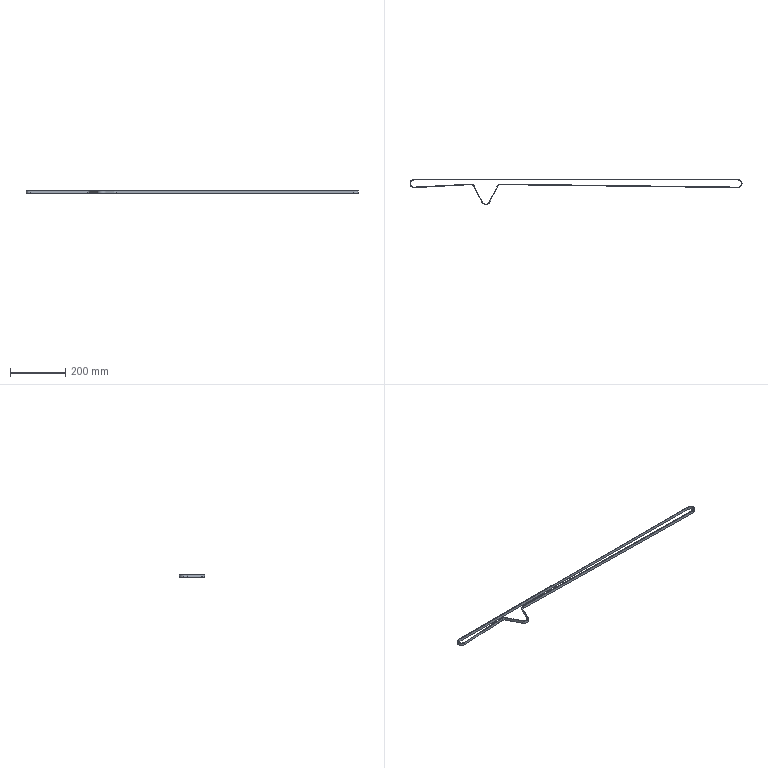Part | STEP file | Timing belt 2505-S3M-10mm wide | 1 solid | 24 faces | box 1199 x 90.84 x 10 mm | volume 50146 mm3 | cylinder 12 | plane 12 | commonest cylinder face diameters 25.68 x3 29.68 x3 20 x2 24 x2 29 x1 33 x1